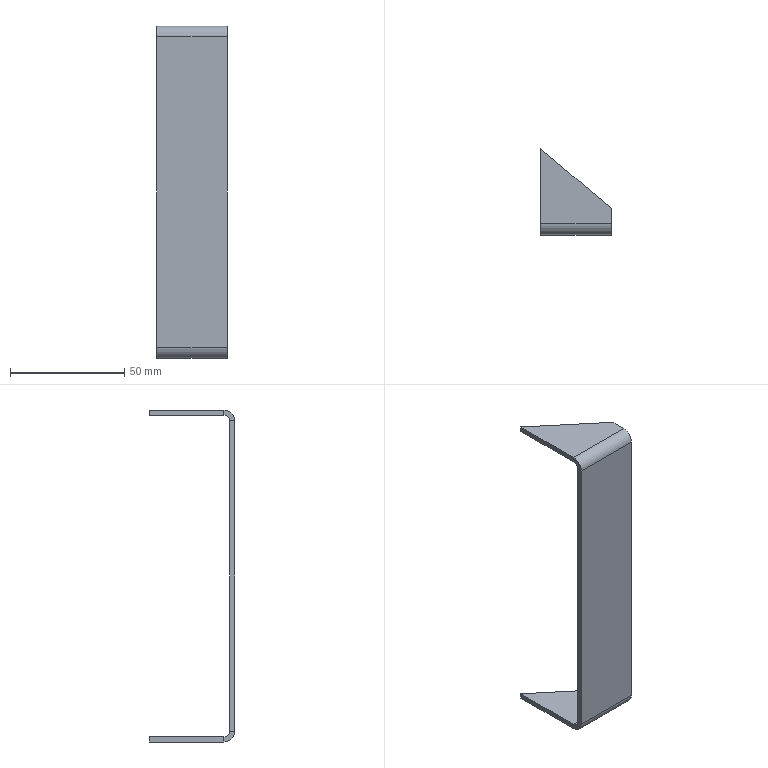Part | SolidWorks | features FlatPattern 1, ICE 1, SMBaseFlange 1, SheetMetal 1 | 1 solid | 22 faces | box 31 x 37.5 x 145 mm | volume 13281 mm3 | plane 18 | cylinder 4 | commonest cylinder face diameters 5 x2 9.6 x2
STEP:
#1=CARTESIAN_POINT('',(15.5,-26.,-2.3));
#2=VERTEX_POINT('',#1);
#3=CARTESIAN_POINT('',(15.5,-32.7,-2.3));
#4=VERTEX_POINT('',#3);
#5=CARTESIAN_POINT('',(15.5,0.,-2.3));
#6=DIRECTION('',(0.,-1.,0.));
#7=VECTOR('',#6,1000.);
#8=LINE('',#5,#7);
#9=EDGE_CURVE('',#2,#4,#8,.T.);
#10=ORIENTED_EDGE('',*,*,#9,.F.);
#11=CARTESIAN_POINT('',(15.5,-26.,0.));
#12=VERTEX_POINT('',#11);
#13=CARTESIAN_POINT('',(15.5,-26.,-2.3));
#14=DIRECTION('',(0.,0.,1.));
#15=VECTOR('',#14,1000.);
#16=LINE('',#13,#15);
#17=EDGE_CURVE('',#2,#12,#16,.T.);
#18=ORIENTED_EDGE('',*,*,#17,.T.);
#19=CARTESIAN_POINT('',(15.5,-32.7,0.));
#20=VERTEX_POINT('',#19);
#21=CARTESIAN_POINT('',(15.5,0.,0.));
#22=DIRECTION('',(0.,-1.,0.));
#23=VECTOR('',#22,1000.);
#24=LINE('',#21,#23);
#25=EDGE_CURVE('',#12,#20,#24,.T.);
#26=ORIENTED_EDGE('',*,*,#25,.T.);
#27=CARTESIAN_POINT('',(15.5,-32.7,0.));
#28=DIRECTION('',(0.,0.,-1.));
#29=VECTOR('',#28,1000.);
#30=LINE('',#27,#29);
#31=EDGE_CURVE('',#20,#4,#30,.T.);
#32=ORIENTED_EDGE('',*,*,#31,.T.);
#33=EDGE_LOOP('',(#10,#18,#26,#32));
#34=FACE_OUTER_BOUND('',#33,.T.);
#35=CARTESIAN_POINT('',(15.5,-35.2,-4.8));
#36=DIRECTION('',(1.,0.,0.));
#37=DIRECTION('',(0.,0.,-1.));
#38=AXIS2_PLACEMENT_3D('',#35,#36,#37);
#39=PLANE('',#38);
#40=ADVANCED_FACE('',(#34),#39,.T.);
#41=CARTESIAN_POINT('',(-15.5,0.,-145.));
#42=VERTEX_POINT('',#41);
#43=CARTESIAN_POINT('',(15.5,-26.,-145.));
#44=VERTEX_POINT('',#43);
#45=CARTESIAN_POINT('',(21.162,-30.749,-145.));
#46=DIRECTION('',(0.7662,-0.6426,0.));
#47=VECTOR('',#46,1000.);
#48=LINE('',#45,#47);
#49=EDGE_CURVE('',#42,#44,#48,.T.);
#50=ORIENTED_EDGE('',*,*,#49,.T.);
#51=CARTESIAN_POINT('',(15.5,-32.7,-145.));
#52=VERTEX_POINT('',#51);
#53=CARTESIAN_POINT('',(15.5,-37.5,-145.));
#54=DIRECTION('',(0.,1.,0.));
#55=VECTOR('',#54,1000.);
#56=LINE('',#53,#55);
#57=EDGE_CURVE('',#52,#44,#56,.T.);
#58=ORIENTED_EDGE('',*,*,#57,.F.);
#59=CARTESIAN_POINT('',(-15.5,-32.7,-145.));
#60=VERTEX_POINT('',#59);
#61=CARTESIAN_POINT('',(15.5,-32.7,-145.));
#62=DIRECTION('',(-1.,0.,0.));
#63=VECTOR('',#62,1000.);
#64=LINE('',#61,#63);
#65=EDGE_CURVE('',#52,#60,#64,.T.);
#66=ORIENTED_EDGE('',*,*,#65,.T.);
#67=CARTESIAN_POINT('',(-15.5,-37.5,-145.));
#68=DIRECTION('',(0.,1.,0.));
#69=VECTOR('',#68,1000.);
#70=LINE('',#67,#69);
#71=EDGE_CURVE('',#60,#42,#70,.T.);
#72=ORIENTED_EDGE('',*,*,#71,.T.);
#73=EDGE_LOOP('',(#50,#58,#66,#72));
#74=FACE_OUTER_BOUND('',#73,.T.);
#75=CARTESIAN_POINT('',(15.5,-37.5,-145.));
#76=DIRECTION('',(0.,0.,1.));
#77=DIRECTION('',(1.,0.,0.));
#78=AXIS2_PLACEMENT_3D('',#75,#76,#77);
#79=PLANE('',#78);
#80=ADVANCED_FACE('',(#74),#79,.F.);
#81=CARTESIAN_POINT('',(15.5,-32.7,-142.7));
#82=VERTEX_POINT('',#81);
#83=CARTESIAN_POINT('',(15.5,-26.,-142.7));
#84=VERTEX_POINT('',#83);
#85=CARTESIAN_POINT('',(15.5,-37.5,-142.7));
#86=DIRECTION('',(0.,1.,0.));
#87=VECTOR('',#86,1000.);
#88=LINE('',#85,#87);
#89=EDGE_CURVE('',#82,#84,#88,.T.);
#90=ORIENTED_EDGE('',*,*,#89,.T.);
#91=CARTESIAN_POINT('',(-15.5,0.,-142.7));
#92=VERTEX_POINT('',#91);
#93=CARTESIAN_POINT('',(21.162,-30.749,-142.7));
#94=DIRECTION('',(0.7662,-0.6426,0.));
#95=VECTOR('',#94,1000.);
#96=LINE('',#93,#95);
#97=EDGE_CURVE('',#92,#84,#96,.T.);
#98=ORIENTED_EDGE('',*,*,#97,.F.);
#99=CARTESIAN_POINT('',(-15.5,-32.7,-142.7));
#100=VERTEX_POINT('',#99);
#101=CARTESIAN_POINT('',(-15.5,-37.5,-142.7));
#102=DIRECTION('',(0.,1.,0.));
#103=VECTOR('',#102,1000.);
#104=LINE('',#101,#103);
#105=EDGE_CURVE('',#100,#92,#104,.T.);
#106=ORIENTED_EDGE('',*,*,#105,.F.);
#107=CARTESIAN_POINT('',(15.5,-32.7,-142.7));
#108=DIRECTION('',(-1.,0.,0.));
#109=VECTOR('',#108,1000.);
#110=LINE('',#107,#109);
#111=EDGE_CURVE('',#82,#100,#110,.T.);
#112=ORIENTED_EDGE('',*,*,#111,.F.);
#113=EDGE_LOOP('',(#90,#98,#106,#112));
#114=FACE_OUTER_BOUND('',#113,.T.);
#115=CARTESIAN_POINT('',(15.5,-37.5,-142.7));
#116=DIRECTION('',(0.,0.,1.));
#117=DIRECTION('',(1.,0.,0.));
#118=AXIS2_PLACEMENT_3D('',#115,#116,#117);
#119=PLANE('',#118);
#120=ADVANCED_FACE('',(#114),#119,.T.);
#121=CARTESIAN_POINT('',(-15.5,0.,-2.3));
#122=VERTEX_POINT('',#121);
#123=CARTESIAN_POINT('',(-15.5,-32.7,-2.3));
#124=VERTEX_POINT('',#123);
#125=CARTESIAN_POINT('',(-15.5,0.,-2.3));
#126=DIRECTION('',(0.,-1.,0.));
#127=VECTOR('',#126,1000.);
#128=LINE('',#125,#127);
#129=EDGE_CURVE('',#122,#124,#128,.T.);
#130=ORIENTED_EDGE('',*,*,#129,.F.);
#131=CARTESIAN_POINT('',(2.699,-15.263,-2.3));
#132=DIRECTION('',(-0.7662,0.6426,0.));
#133=VECTOR('',#132,1000.);
#134=LINE('',#131,#133);
#135=EDGE_CURVE('',#2,#122,#134,.T.);
#136=ORIENTED_EDGE('',*,*,#135,.F.);
#137=ORIENTED_EDGE('',*,*,#9,.T.);
#138=CARTESIAN_POINT('',(15.5,-32.7,-2.3));
#139=DIRECTION('',(-1.,0.,0.));
#140=VECTOR('',#139,1000.);
#141=LINE('',#138,#140);
#142=EDGE_CURVE('',#4,#124,#141,.T.);
#143=ORIENTED_EDGE('',*,*,#142,.T.);
#144=EDGE_LOOP('',(#130,#136,#137,#143));
#145=FACE_OUTER_BOUND('',#144,.T.);
#146=CARTESIAN_POINT('',(15.5,0.,-2.3));
#147=DIRECTION('',(0.,0.,-1.));
#148=DIRECTION('',(0.,1.,0.));
#149=AXIS2_PLACEMENT_3D('',#146,#147,#148);
#150=PLANE('',#149);
#151=ADVANCED_FACE('',(#145),#150,.T.);
#152=CARTESIAN_POINT('',(-15.5,0.,0.));
#153=VERTEX_POINT('',#152);
#154=CARTESIAN_POINT('',(2.699,-15.263,0.));
#155=DIRECTION('',(-0.7662,0.6426,0.));
#156=VECTOR('',#155,1000.);
#157=LINE('',#154,#156);
#158=EDGE_CURVE('',#12,#153,#157,.T.);
#159=ORIENTED_EDGE('',*,*,#158,.T.);
#160=CARTESIAN_POINT('',(-15.5,-32.7,0.));
#161=VERTEX_POINT('',#160);
#162=CARTESIAN_POINT('',(-15.5,0.,0.));
#163=DIRECTION('',(0.,-1.,0.));
#164=VECTOR('',#163,1000.);
#165=LINE('',#162,#164);
#166=EDGE_CURVE('',#153,#161,#165,.T.);
#167=ORIENTED_EDGE('',*,*,#166,.T.);
#168=CARTESIAN_POINT('',(15.5,-32.7,0.));
#169=DIRECTION('',(-1.,0.,0.));
#170=VECTOR('',#169,1000.);
#171=LINE('',#168,#170);
#172=EDGE_CURVE('',#20,#161,#171,.T.);
#173=ORIENTED_EDGE('',*,*,#172,.F.);
#174=ORIENTED_EDGE('',*,*,#25,.F.);
#175=EDGE_LOOP('',(#159,#167,#173,#174));
#176=FACE_OUTER_BOUND('',#175,.T.);
#177=CARTESIAN_POINT('',(15.5,0.,0.));
#178=DIRECTION('',(0.,0.,-1.));
#179=DIRECTION('',(0.,1.,0.));
#180=AXIS2_PLACEMENT_3D('',#177,#178,#179);
#181=PLANE('',#180);
#182=ADVANCED_FACE('',(#176),#181,.F.);
#183=ORIENTED_EDGE('',*,*,#57,.T.);
#184=CARTESIAN_POINT('',(15.5,-26.,-142.7));
#185=DIRECTION('',(0.,0.,-1.));
#186=VECTOR('',#185,1000.);
#187=LINE('',#184,#186);
#188=EDGE_CURVE('',#84,#44,#187,.T.);
#189=ORIENTED_EDGE('',*,*,#188,.F.);
#190=ORIENTED_EDGE('',*,*,#89,.F.);
#191=CARTESIAN_POINT('',(15.5,-32.7,-142.7));
#192=DIRECTION('',(0.,0.,-1.));
#193=VECTOR('',#192,1000.);
#194=LINE('',#191,#193);
#195=EDGE_CURVE('',#82,#52,#194,.T.);
#196=ORIENTED_EDGE('',*,*,#195,.T.);
#197=EDGE_LOOP('',(#183,#189,#190,#196));
#198=FACE_OUTER_BOUND('',#197,.T.);
#199=CARTESIAN_POINT('',(15.5,-32.7,-140.2));
#200=DIRECTION('',(1.,0.,0.));
#201=DIRECTION('',(0.,0.,-1.));
#202=AXIS2_PLACEMENT_3D('',#199,#200,#201);
#203=PLANE('',#202);
#204=ADVANCED_FACE('',(#198),#203,.T.);
#205=ORIENTED_EDGE('',*,*,#31,.F.);
#206=CARTESIAN_POINT('',(15.5,-37.5,-4.8));
#207=VERTEX_POINT('',#206);
#208=CARTESIAN_POINT('',(15.5,-32.7,-4.8));
#209=DIRECTION('',(1.,0.,0.));
#210=DIRECTION('',(0.,0.,1.));
#211=AXIS2_PLACEMENT_3D('',#208,#209,#210);
#212=CIRCLE('',#211,4.8);
#213=EDGE_CURVE('',#20,#207,#212,.T.);
#214=ORIENTED_EDGE('',*,*,#213,.T.);
#215=CARTESIAN_POINT('',(15.5,-35.2,-4.8));
#216=VERTEX_POINT('',#215);
#217=CARTESIAN_POINT('',(15.5,-35.2,-4.8));
#218=DIRECTION('',(0.,-1.,0.));
#219=VECTOR('',#218,1000.);
#220=LINE('',#217,#219);
#221=EDGE_CURVE('',#216,#207,#220,.T.);
#222=ORIENTED_EDGE('',*,*,#221,.F.);
#223=CARTESIAN_POINT('',(15.5,-32.7,-4.8));
#224=DIRECTION('',(1.,0.,0.));
#225=DIRECTION('',(0.,0.,-1.));
#226=AXIS2_PLACEMENT_3D('',#223,#224,#225);
#227=CIRCLE('',#226,2.5);
#228=EDGE_CURVE('',#4,#216,#227,.T.);
#229=ORIENTED_EDGE('',*,*,#228,.F.);
#230=EDGE_LOOP('',(#205,#214,#222,#229));
#231=FACE_OUTER_BOUND('',#230,.T.);
#232=CARTESIAN_POINT('',(15.5,-32.7,0.));
#233=DIRECTION('',(1.,0.,0.));
#234=DIRECTION('',(0.,0.,-1.));
#235=AXIS2_PLACEMENT_3D('',#232,#233,#234);
#236=PLANE('',#235);
#237=ADVANCED_FACE('',(#231),#236,.T.);
#238=CARTESIAN_POINT('',(-15.5,-37.5,-4.8));
#239=VERTEX_POINT('',#238);
#240=CARTESIAN_POINT('',(-15.5,-35.2,-4.8));
#241=VERTEX_POINT('',#240);
#242=CARTESIAN_POINT('',(-15.5,-37.5,-4.8));
#243=DIRECTION('',(0.,1.,0.));
#244=VECTOR('',#243,1000.);
#245=LINE('',#242,#244);
#246=EDGE_CURVE('',#239,#241,#245,.T.);
#247=ORIENTED_EDGE('',*,*,#246,.F.);
#248=CARTESIAN_POINT('',(-15.5,-32.7,-4.8));
#249=DIRECTION('',(1.,0.,0.));
#250=DIRECTION('',(0.,0.,1.));
#251=AXIS2_PLACEMENT_3D('',#248,#249,#250);
#252=CIRCLE('',#251,4.8);
#253=EDGE_CURVE('',#161,#239,#252,.T.);
#254=ORIENTED_EDGE('',*,*,#253,.F.);
#255=CARTESIAN_POINT('',(-15.5,-32.7,-2.3));
#256=DIRECTION('',(0.,0.,1.));
#257=VECTOR('',#256,1000.);
#258=LINE('',#255,#257);
#259=EDGE_CURVE('',#124,#161,#258,.T.);
#260=ORIENTED_EDGE('',*,*,#259,.F.);
#261=CARTESIAN_POINT('',(-15.5,-32.7,-4.8));
#262=DIRECTION('',(1.,0.,0.));
#263=DIRECTION('',(0.,0.,-1.));
#264=AXIS2_PLACEMENT_3D('',#261,#262,#263);
#265=CIRCLE('',#264,2.5);
#266=EDGE_CURVE('',#124,#241,#265,.T.);
#267=ORIENTED_EDGE('',*,*,#266,.T.);
#268=EDGE_LOOP('',(#247,#254,#260,#267));
#269=FACE_OUTER_BOUND('',#268,.T.);
#270=CARTESIAN_POINT('',(-15.5,-37.5,-4.8));
#271=DIRECTION('',(-1.,0.,0.));
#272=DIRECTION('',(0.,0.,1.));
#273=AXIS2_PLACEMENT_3D('',#270,#271,#272);
#274=PLANE('',#273);
#275=ADVANCED_FACE('',(#269),#274,.T.);
#276=CARTESIAN_POINT('',(-15.5,-37.5,-140.2));
#277=VERTEX_POINT('',#276);
#278=CARTESIAN_POINT('',(-15.5,-37.5,0.));
#279=DIRECTION('',(0.,0.,-1.));
#280=VECTOR('',#279,1000.);
#281=LINE('',#278,#280);
#282=EDGE_CURVE('',#239,#277,#281,.T.);
#283=ORIENTED_EDGE('',*,*,#282,.F.);
#284=ORIENTED_EDGE('',*,*,#246,.T.);
#285=CARTESIAN_POINT('',(-15.5,-35.2,-140.2));
#286=VERTEX_POINT('',#285);
#287=CARTESIAN_POINT('',(-15.5,-35.2,0.));
#288=DIRECTION('',(0.,0.,-1.));
#289=VECTOR('',#288,1000.);
#290=LINE('',#287,#289);
#291=EDGE_CURVE('',#241,#286,#290,.T.);
#292=ORIENTED_EDGE('',*,*,#291,.T.);
#293=CARTESIAN_POINT('',(-15.5,-35.2,-140.2));
#294=DIRECTION('',(0.,-1.,0.));
#295=VECTOR('',#294,1000.);
#296=LINE('',#293,#295);
#297=EDGE_CURVE('',#286,#277,#296,.T.);
#298=ORIENTED_EDGE('',*,*,#297,.T.);
#299=EDGE_LOOP('',(#283,#284,#292,#298));
#300=FACE_OUTER_BOUND('',#299,.T.);
#301=CARTESIAN_POINT('',(-15.5,-32.7,-2.3));
#302=DIRECTION('',(-1.,0.,0.));
#303=DIRECTION('',(0.,0.,1.));
#304=AXIS2_PLACEMENT_3D('',#301,#302,#303);
#305=PLANE('',#304);
#306=ADVANCED_FACE('',(#300),#305,.T.);
#307=CARTESIAN_POINT('',(15.5,-37.5,-140.2));
#308=VERTEX_POINT('',#307);
#309=CARTESIAN_POINT('',(15.5,-35.2,-140.2));
#310=VERTEX_POINT('',#309);
#311=CARTESIAN_POINT('',(15.5,-37.5,-140.2));
#312=DIRECTION('',(0.,1.,0.));
#313=VECTOR('',#312,1000.);
#314=LINE('',#311,#313);
#315=EDGE_CURVE('',#308,#310,#314,.T.);
#316=ORIENTED_EDGE('',*,*,#315,.F.);
#317=CARTESIAN_POINT('',(15.5,-32.7,-140.2));
#318=DIRECTION('',(1.,0.,0.));
#319=DIRECTION('',(0.,0.,1.));
#320=AXIS2_PLACEMENT_3D('',#317,#318,#319);
#321=CIRCLE('',#320,4.8);
#322=EDGE_CURVE('',#308,#52,#321,.T.);
#323=ORIENTED_EDGE('',*,*,#322,.T.);
#324=ORIENTED_EDGE('',*,*,#195,.F.);
#325=CARTESIAN_POINT('',(15.5,-32.7,-140.2));
#326=DIRECTION('',(1.,0.,0.));
#327=DIRECTION('',(0.,0.,-1.));
#328=AXIS2_PLACEMENT_3D('',#325,#326,#327);
#329=CIRCLE('',#328,2.5);
#330=EDGE_CURVE('',#310,#82,#329,.T.);
#331=ORIENTED_EDGE('',*,*,#330,.F.);
#332=EDGE_LOOP('',(#316,#323,#324,#331));
#333=FACE_OUTER_BOUND('',#332,.T.);
#334=CARTESIAN_POINT('',(15.5,-37.5,-140.2));
#335=DIRECTION('',(1.,0.,0.));
#336=DIRECTION('',(0.,0.,-1.));
#337=AXIS2_PLACEMENT_3D('',#334,#335,#336);
#338=PLANE('',#337);
#339=ADVANCED_FACE('',(#333),#338,.T.);
#340=CARTESIAN_POINT('',(15.5,-37.5,0.));
#341=DIRECTION('',(0.,0.,-1.));
#342=VECTOR('',#341,1000.);
#343=LINE('',#340,#342);
#344=EDGE_CURVE('',#207,#308,#343,.T.);
#345=ORIENTED_EDGE('',*,*,#344,.T.);
#346=ORIENTED_EDGE('',*,*,#315,.T.);
#347=CARTESIAN_POINT('',(15.5,-35.2,0.));
#348=DIRECTION('',(0.,0.,-1.));
#349=VECTOR('',#348,1000.);
#350=LINE('',#347,#349);
#351=EDGE_CURVE('',#216,#310,#350,.T.);
#352=ORIENTED_EDGE('',*,*,#351,.F.);
#353=ORIENTED_EDGE('',*,*,#221,.T.);
#354=EDGE_LOOP('',(#345,#346,#352,#353));
#355=FACE_OUTER_BOUND('',#354,.T.);
#356=CARTESIAN_POINT('',(15.5,-32.7,-142.7));
#357=DIRECTION('',(1.,0.,0.));
#358=DIRECTION('',(0.,0.,-1.));
#359=AXIS2_PLACEMENT_3D('',#356,#357,#358);
#360=PLANE('',#359);
#361=ADVANCED_FACE('',(#355),#360,.T.);
#362=CARTESIAN_POINT('',(-15.5,-32.7,-145.));
#363=DIRECTION('',(0.,0.,1.));
#364=VECTOR('',#363,1000.);
#365=LINE('',#362,#364);
#366=EDGE_CURVE('',#60,#100,#365,.T.);
#367=ORIENTED_EDGE('',*,*,#366,.F.);
#368=CARTESIAN_POINT('',(-15.5,-32.7,-140.2));
#369=DIRECTION('',(1.,0.,0.));
#370=DIRECTION('',(0.,0.,1.));
#371=AXIS2_PLACEMENT_3D('',#368,#369,#370);
#372=CIRCLE('',#371,4.8);
#373=EDGE_CURVE('',#277,#60,#372,.T.);
#374=ORIENTED_EDGE('',*,*,#373,.F.);
#375=ORIENTED_EDGE('',*,*,#297,.F.);
#376=CARTESIAN_POINT('',(-15.5,-32.7,-140.2));
#377=DIRECTION('',(1.,0.,0.));
#378=DIRECTION('',(0.,0.,-1.));
#379=AXIS2_PLACEMENT_3D('',#376,#377,#378);
#380=CIRCLE('',#379,2.5);
#381=EDGE_CURVE('',#286,#100,#380,.T.);
#382=ORIENTED_EDGE('',*,*,#381,.T.);
#383=EDGE_LOOP('',(#367,#374,#375,#382));
#384=FACE_OUTER_BOUND('',#383,.T.);
#385=CARTESIAN_POINT('',(-15.5,-32.7,-145.));
#386=DIRECTION('',(-1.,0.,0.));
#387=DIRECTION('',(0.,0.,1.));
#388=AXIS2_PLACEMENT_3D('',#385,#386,#387);
#389=PLANE('',#388);
#390=ADVANCED_FACE('',(#384),#389,.T.);
#391=ORIENTED_EDGE('',*,*,#71,.F.);
#392=ORIENTED_EDGE('',*,*,#366,.T.);
#393=ORIENTED_EDGE('',*,*,#105,.T.);
#394=CARTESIAN_POINT('',(-15.5,0.,-142.7));
#395=DIRECTION('',(0.,0.,-1.));
#396=VECTOR('',#395,1000.);
#397=LINE('',#394,#396);
#398=EDGE_CURVE('',#92,#42,#397,.T.);
#399=ORIENTED_EDGE('',*,*,#398,.T.);
#400=EDGE_LOOP('',(#391,#392,#393,#399));
#401=FACE_OUTER_BOUND('',#400,.T.);
#402=CARTESIAN_POINT('',(-15.5,-35.2,-140.2));
#403=DIRECTION('',(-1.,0.,0.));
#404=DIRECTION('',(0.,0.,1.));
#405=AXIS2_PLACEMENT_3D('',#402,#403,#404);
#406=PLANE('',#405);
#407=ADVANCED_FACE('',(#401),#406,.T.);
#408=ORIENTED_EDGE('',*,*,#381,.F.);
#409=CARTESIAN_POINT('',(15.5,-35.2,-140.2));
#410=DIRECTION('',(-1.,0.,0.));
#411=VECTOR('',#410,1000.);
#412=LINE('',#409,#411);
#413=EDGE_CURVE('',#310,#286,#412,.T.);
#414=ORIENTED_EDGE('',*,*,#413,.F.);
#415=ORIENTED_EDGE('',*,*,#330,.T.);
#416=ORIENTED_EDGE('',*,*,#111,.T.);
#417=EDGE_LOOP('',(#408,#414,#415,#416));
#418=FACE_OUTER_BOUND('',#417,.T.);
#419=CARTESIAN_POINT('',(15.5,-32.7,-140.2));
#420=DIRECTION('',(-1.,0.,0.));
#421=DIRECTION('',(0.,0.,1.));
#422=AXIS2_PLACEMENT_3D('',#419,#420,#421);
#423=CYLINDRICAL_SURFACE('',#422,2.5);
#424=ADVANCED_FACE('',(#418),#423,.F.);
#425=ORIENTED_EDGE('',*,*,#291,.F.);
#426=CARTESIAN_POINT('',(15.5,-35.2,-4.8));
#427=DIRECTION('',(-1.,0.,0.));
#428=VECTOR('',#427,1000.);
#429=LINE('',#426,#428);
#430=EDGE_CURVE('',#216,#241,#429,.T.);
#431=ORIENTED_EDGE('',*,*,#430,.F.);
#432=ORIENTED_EDGE('',*,*,#351,.T.);
#433=ORIENTED_EDGE('',*,*,#413,.T.);
#434=EDGE_LOOP('',(#425,#431,#432,#433));
#435=FACE_OUTER_BOUND('',#434,.T.);
#436=CARTESIAN_POINT('',(15.5,-35.2,0.));
#437=DIRECTION('',(0.,1.,0.));
#438=DIRECTION('',(0.,0.,1.));
#439=AXIS2_PLACEMENT_3D('',#436,#437,#438);
#440=PLANE('',#439);
#441=ADVANCED_FACE('',(#435),#440,.T.);
#442=ORIENTED_EDGE('',*,*,#266,.F.);
#443=ORIENTED_EDGE('',*,*,#142,.F.);
#444=ORIENTED_EDGE('',*,*,#228,.T.);
#445=ORIENTED_EDGE('',*,*,#430,.T.);
#446=EDGE_LOOP('',(#442,#443,#444,#445));
#447=FACE_OUTER_BOUND('',#446,.T.);
#448=CARTESIAN_POINT('',(15.5,-32.7,-4.8));
#449=DIRECTION('',(-1.,0.,0.));
#450=DIRECTION('',(0.,0.,1.));
#451=AXIS2_PLACEMENT_3D('',#448,#449,#450);
#452=CYLINDRICAL_SURFACE('',#451,2.5);
#453=ADVANCED_FACE('',(#447),#452,.F.);
#454=ORIENTED_EDGE('',*,*,#253,.T.);
#455=CARTESIAN_POINT('',(15.5,-37.5,-4.8));
#456=DIRECTION('',(-1.,0.,0.));
#457=VECTOR('',#456,1000.);
#458=LINE('',#455,#457);
#459=EDGE_CURVE('',#207,#239,#458,.T.);
#460=ORIENTED_EDGE('',*,*,#459,.F.);
#461=ORIENTED_EDGE('',*,*,#213,.F.);
#462=ORIENTED_EDGE('',*,*,#172,.T.);
#463=EDGE_LOOP('',(#454,#460,#461,#462));
#464=FACE_OUTER_BOUND('',#463,.T.);
#465=CARTESIAN_POINT('',(15.5,-32.7,-4.8));
#466=DIRECTION('',(-1.,0.,0.));
#467=DIRECTION('',(0.,0.,1.));
#468=AXIS2_PLACEMENT_3D('',#465,#466,#467);
#469=CYLINDRICAL_SURFACE('',#468,4.8);
#470=ADVANCED_FACE('',(#464),#469,.T.);
#471=ORIENTED_EDGE('',*,*,#282,.T.);
#472=CARTESIAN_POINT('',(15.5,-37.5,-140.2));
#473=DIRECTION('',(-1.,0.,0.));
#474=VECTOR('',#473,1000.);
#475=LINE('',#472,#474);
#476=EDGE_CURVE('',#308,#277,#475,.T.);
#477=ORIENTED_EDGE('',*,*,#476,.F.);
#478=ORIENTED_EDGE('',*,*,#344,.F.);
#479=ORIENTED_EDGE('',*,*,#459,.T.);
#480=EDGE_LOOP('',(#471,#477,#478,#479));
#481=FACE_OUTER_BOUND('',#480,.T.);
#482=CARTESIAN_POINT('',(15.5,-37.5,0.));
#483=DIRECTION('',(0.,1.,0.));
#484=DIRECTION('',(0.,0.,1.));
#485=AXIS2_PLACEMENT_3D('',#482,#483,#484);
#486=PLANE('',#485);
#487=ADVANCED_FACE('',(#481),#486,.F.);
#488=ORIENTED_EDGE('',*,*,#373,.T.);
#489=ORIENTED_EDGE('',*,*,#65,.F.);
#490=ORIENTED_EDGE('',*,*,#322,.F.);
#491=ORIENTED_EDGE('',*,*,#476,.T.);
#492=EDGE_LOOP('',(#488,#489,#490,#491));
#493=FACE_OUTER_BOUND('',#492,.T.);
#494=CARTESIAN_POINT('',(15.5,-32.7,-140.2));
#495=DIRECTION('',(-1.,0.,0.));
#496=DIRECTION('',(0.,0.,1.));
#497=AXIS2_PLACEMENT_3D('',#494,#495,#496);
#498=CYLINDRICAL_SURFACE('',#497,4.8);
#499=ADVANCED_FACE('',(#493),#498,.T.);
#500=ORIENTED_EDGE('',*,*,#129,.T.);
#501=ORIENTED_EDGE('',*,*,#259,.T.);
#502=ORIENTED_EDGE('',*,*,#166,.F.);
#503=CARTESIAN_POINT('',(-15.5,0.,0.));
#504=DIRECTION('',(0.,0.,-1.));
#505=VECTOR('',#504,1000.);
#506=LINE('',#503,#505);
#507=EDGE_CURVE('',#153,#122,#506,.T.);
#508=ORIENTED_EDGE('',*,*,#507,.T.);
#509=EDGE_LOOP('',(#500,#501,#502,#508));
#510=FACE_OUTER_BOUND('',#509,.T.);
#511=CARTESIAN_POINT('',(-15.5,-32.7,-140.2));
#512=DIRECTION('',(1.,0.,0.));
#513=DIRECTION('',(0.,0.,-1.));
#514=AXIS2_PLACEMENT_3D('',#511,#512,#513);
#515=PLANE('',#514);
#516=ADVANCED_FACE('',(#510),#515,.F.);
#517=ORIENTED_EDGE('',*,*,#135,.T.);
#518=ORIENTED_EDGE('',*,*,#507,.F.);
#519=ORIENTED_EDGE('',*,*,#158,.F.);
#520=ORIENTED_EDGE('',*,*,#17,.F.);
#521=EDGE_LOOP('',(#517,#518,#519,#520));
#522=FACE_OUTER_BOUND('',#521,.T.);
#523=CARTESIAN_POINT('',(2.699,-15.263,-2.3));
#524=DIRECTION('',(-0.6426,-0.7662,0.));
#525=DIRECTION('',(-0.7662,0.6426,0.));
#526=AXIS2_PLACEMENT_3D('',#523,#524,#525);
#527=PLANE('',#526);
#528=ADVANCED_FACE('',(#522),#527,.F.);
#529=ORIENTED_EDGE('',*,*,#97,.T.);
#530=ORIENTED_EDGE('',*,*,#188,.T.);
#531=ORIENTED_EDGE('',*,*,#49,.F.);
#532=ORIENTED_EDGE('',*,*,#398,.F.);
#533=EDGE_LOOP('',(#529,#530,#531,#532));
#534=FACE_OUTER_BOUND('',#533,.T.);
#535=CARTESIAN_POINT('',(21.162,-30.749,-142.7));
#536=DIRECTION('',(-0.6426,-0.7662,0.));
#537=DIRECTION('',(0.7662,-0.6426,0.));
#538=AXIS2_PLACEMENT_3D('',#535,#536,#537);
#539=PLANE('',#538);
#540=ADVANCED_FACE('',(#534),#539,.F.);
#541=CLOSED_SHELL('',(#40,#80,#120,#151,#182,#204,#237,#275,#306,#339,#361,#390,#407,#424,#441,#453,#470,#487,#499,#516,#528,#540));
#542=MANIFOLD_SOLID_BREP('',#541);
#543=CARTESIAN_POINT('',(0.,0.,0.));
#544=DIRECTION('',(0.,0.,1.));
#545=DIRECTION('',(1.,0.,0.));
#546=AXIS2_PLACEMENT_3D('',#543,#544,#545);
#547=(LENGTH_UNIT()NAMED_UNIT(*)SI_UNIT(.MILLI.,.METRE.));
#548=UNCERTAINTY_MEASURE_WITH_UNIT(LENGTH_MEASURE(0.00001),#547,'','');
#549=(NAMED_UNIT(*)PLANE_ANGLE_UNIT()SI_UNIT($,.RADIAN.));
#550=(NAMED_UNIT(*)SI_UNIT($,.STERADIAN.)SOLID_ANGLE_UNIT());
#551=(GEOMETRIC_REPRESENTATION_CONTEXT(3)GLOBAL_UNCERTAINTY_ASSIGNED_CONTEXT((#548))GLOBAL_UNIT_ASSIGNED_CONTEXT((#547,#549,#550))REPRESENTATION_CONTEXT('',''));
#552=ADVANCED_BREP_SHAPE_REPRESENTATION('',(#542,#546),#551);